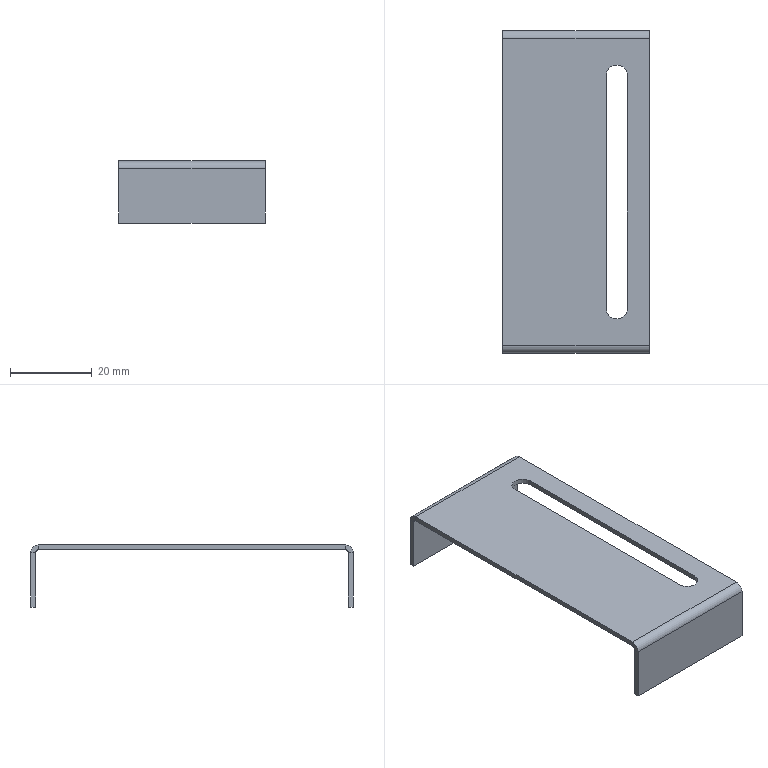Part | 1 solid | 26 faces | box 36 x 79 x 15.2 mm | volume 4192 mm3 | plane 20 | cylinder 6 | commonest cylinder face diameters 1.473 x2 3.873 x2 5.2 x2
STEP:
#1=CARTESIAN_POINT('',(12.6,-28.5,-1.2));
#2=VERTEX_POINT('',#1);
#3=CARTESIAN_POINT('',(7.4,-28.5,-1.2));
#4=VERTEX_POINT('',#3);
#5=CARTESIAN_POINT('',(10.,-28.5,-1.2));
#6=DIRECTION('',(0.,0.,-1.));
#7=DIRECTION('',(-1.,0.,0.));
#8=AXIS2_PLACEMENT_3D('',#5,#6,#7);
#9=CIRCLE('',#8,2.6);
#10=EDGE_CURVE('',#2,#4,#9,.T.);
#11=ORIENTED_EDGE('',*,*,#10,.F.);
#12=CARTESIAN_POINT('',(12.6,28.5,-1.2));
#13=VERTEX_POINT('',#12);
#14=CARTESIAN_POINT('',(12.6,-28.5,-1.2));
#15=DIRECTION('',(0.,-1.,0.));
#16=VECTOR('',#15,1000.);
#17=LINE('',#14,#16);
#18=EDGE_CURVE('',#13,#2,#17,.T.);
#19=ORIENTED_EDGE('',*,*,#18,.F.);
#20=CARTESIAN_POINT('',(7.4,28.5,-1.2));
#21=VERTEX_POINT('',#20);
#22=CARTESIAN_POINT('',(10.,28.5,-1.2));
#23=DIRECTION('',(0.,0.,-1.));
#24=DIRECTION('',(-1.,0.,0.));
#25=AXIS2_PLACEMENT_3D('',#22,#23,#24);
#26=CIRCLE('',#25,2.6);
#27=EDGE_CURVE('',#21,#13,#26,.T.);
#28=ORIENTED_EDGE('',*,*,#27,.F.);
#29=CARTESIAN_POINT('',(7.4,-28.5,-1.2));
#30=DIRECTION('',(0.,1.,0.));
#31=VECTOR('',#30,1000.);
#32=LINE('',#29,#31);
#33=EDGE_CURVE('',#4,#21,#32,.T.);
#34=ORIENTED_EDGE('',*,*,#33,.F.);
#35=EDGE_LOOP('',(#11,#19,#28,#34));
#36=FACE_BOUND('',#35,.T.);
#37=CARTESIAN_POINT('',(18.,-37.563,-1.2));
#38=VERTEX_POINT('',#37);
#39=CARTESIAN_POINT('',(18.,37.563,-1.2));
#40=VERTEX_POINT('',#39);
#41=CARTESIAN_POINT('',(18.,-39.5,-1.2));
#42=DIRECTION('',(0.,1.,0.));
#43=VECTOR('',#42,1000.);
#44=LINE('',#41,#43);
#45=EDGE_CURVE('',#38,#40,#44,.T.);
#46=ORIENTED_EDGE('',*,*,#45,.F.);
#47=CARTESIAN_POINT('',(-18.,-37.563,-1.2));
#48=VERTEX_POINT('',#47);
#49=CARTESIAN_POINT('',(-18.,-37.563,-1.2));
#50=DIRECTION('',(1.,0.,0.));
#51=VECTOR('',#50,1000.);
#52=LINE('',#49,#51);
#53=EDGE_CURVE('',#48,#38,#52,.T.);
#54=ORIENTED_EDGE('',*,*,#53,.F.);
#55=CARTESIAN_POINT('',(-18.,37.563,-1.2));
#56=VERTEX_POINT('',#55);
#57=CARTESIAN_POINT('',(-18.,-39.5,-1.2));
#58=DIRECTION('',(0.,-1.,0.));
#59=VECTOR('',#58,1000.);
#60=LINE('',#57,#59);
#61=EDGE_CURVE('',#56,#48,#60,.T.);
#62=ORIENTED_EDGE('',*,*,#61,.F.);
#63=CARTESIAN_POINT('',(18.,37.563,-1.2));
#64=DIRECTION('',(-1.,0.,0.));
#65=VECTOR('',#64,1000.);
#66=LINE('',#63,#65);
#67=EDGE_CURVE('',#40,#56,#66,.T.);
#68=ORIENTED_EDGE('',*,*,#67,.F.);
#69=EDGE_LOOP('',(#46,#54,#62,#68));
#70=FACE_OUTER_BOUND('',#69,.T.);
#71=CARTESIAN_POINT('',(0.,0.,-1.2));
#72=DIRECTION('',(0.,0.,-1.));
#73=DIRECTION('',(-1.,0.,0.));
#74=AXIS2_PLACEMENT_3D('',#71,#72,#73);
#75=PLANE('',#74);
#76=ADVANCED_FACE('',(#36,#70),#75,.T.);
#77=CARTESIAN_POINT('',(12.6,28.5,0.));
#78=VERTEX_POINT('',#77);
#79=CARTESIAN_POINT('',(12.6,-28.5,0.));
#80=VERTEX_POINT('',#79);
#81=CARTESIAN_POINT('',(12.6,0.,0.));
#82=DIRECTION('',(0.,-1.,0.));
#83=VECTOR('',#82,1000.);
#84=LINE('',#81,#83);
#85=EDGE_CURVE('',#78,#80,#84,.T.);
#86=ORIENTED_EDGE('',*,*,#85,.T.);
#87=CARTESIAN_POINT('',(7.4,-28.5,0.));
#88=VERTEX_POINT('',#87);
#89=CARTESIAN_POINT('',(10.,-28.5,0.));
#90=DIRECTION('',(0.,0.,-1.));
#91=DIRECTION('',(-1.,0.,0.));
#92=AXIS2_PLACEMENT_3D('',#89,#90,#91);
#93=CIRCLE('',#92,2.6);
#94=EDGE_CURVE('',#80,#88,#93,.T.);
#95=ORIENTED_EDGE('',*,*,#94,.T.);
#96=CARTESIAN_POINT('',(7.4,28.5,0.));
#97=VERTEX_POINT('',#96);
#98=CARTESIAN_POINT('',(7.4,0.,0.));
#99=DIRECTION('',(0.,1.,0.));
#100=VECTOR('',#99,1000.);
#101=LINE('',#98,#100);
#102=EDGE_CURVE('',#88,#97,#101,.T.);
#103=ORIENTED_EDGE('',*,*,#102,.T.);
#104=CARTESIAN_POINT('',(10.,28.5,0.));
#105=DIRECTION('',(0.,0.,-1.));
#106=DIRECTION('',(-1.,0.,0.));
#107=AXIS2_PLACEMENT_3D('',#104,#105,#106);
#108=CIRCLE('',#107,2.6);
#109=EDGE_CURVE('',#97,#78,#108,.T.);
#110=ORIENTED_EDGE('',*,*,#109,.T.);
#111=EDGE_LOOP('',(#86,#95,#103,#110));
#112=FACE_BOUND('',#111,.T.);
#113=CARTESIAN_POINT('',(-18.,-37.563,0.));
#114=VERTEX_POINT('',#113);
#115=CARTESIAN_POINT('',(18.,-37.563,0.));
#116=VERTEX_POINT('',#115);
#117=CARTESIAN_POINT('',(-18.,-37.563,0.));
#118=DIRECTION('',(1.,0.,0.));
#119=VECTOR('',#118,1000.);
#120=LINE('',#117,#119);
#121=EDGE_CURVE('',#114,#116,#120,.T.);
#122=ORIENTED_EDGE('',*,*,#121,.T.);
#123=CARTESIAN_POINT('',(18.,37.563,0.));
#124=VERTEX_POINT('',#123);
#125=CARTESIAN_POINT('',(18.,-39.5,0.));
#126=DIRECTION('',(0.,1.,0.));
#127=VECTOR('',#126,1000.);
#128=LINE('',#125,#127);
#129=EDGE_CURVE('',#116,#124,#128,.T.);
#130=ORIENTED_EDGE('',*,*,#129,.T.);
#131=CARTESIAN_POINT('',(-18.,37.563,0.));
#132=VERTEX_POINT('',#131);
#133=CARTESIAN_POINT('',(18.,37.563,0.));
#134=DIRECTION('',(-1.,0.,0.));
#135=VECTOR('',#134,1000.);
#136=LINE('',#133,#135);
#137=EDGE_CURVE('',#124,#132,#136,.T.);
#138=ORIENTED_EDGE('',*,*,#137,.T.);
#139=CARTESIAN_POINT('',(-18.,-39.5,0.));
#140=DIRECTION('',(0.,-1.,0.));
#141=VECTOR('',#140,1000.);
#142=LINE('',#139,#141);
#143=EDGE_CURVE('',#132,#114,#142,.T.);
#144=ORIENTED_EDGE('',*,*,#143,.T.);
#145=EDGE_LOOP('',(#122,#130,#138,#144));
#146=FACE_OUTER_BOUND('',#145,.T.);
#147=CARTESIAN_POINT('',(0.,0.,0.));
#148=DIRECTION('',(0.,0.,-1.));
#149=DIRECTION('',(-1.,0.,0.));
#150=AXIS2_PLACEMENT_3D('',#147,#148,#149);
#151=PLANE('',#150);
#152=ADVANCED_FACE('',(#112,#146),#151,.F.);
#153=ORIENTED_EDGE('',*,*,#61,.T.);
#154=CARTESIAN_POINT('',(-18.,-37.563,-1.2));
#155=DIRECTION('',(0.,0.,1.));
#156=VECTOR('',#155,1000.);
#157=LINE('',#154,#156);
#158=EDGE_CURVE('',#48,#114,#157,.T.);
#159=ORIENTED_EDGE('',*,*,#158,.T.);
#160=ORIENTED_EDGE('',*,*,#143,.F.);
#161=CARTESIAN_POINT('',(-18.,37.563,-1.2));
#162=DIRECTION('',(0.,0.,1.));
#163=VECTOR('',#162,1000.);
#164=LINE('',#161,#163);
#165=EDGE_CURVE('',#56,#132,#164,.T.);
#166=ORIENTED_EDGE('',*,*,#165,.F.);
#167=EDGE_LOOP('',(#153,#159,#160,#166));
#168=FACE_OUTER_BOUND('',#167,.T.);
#169=CARTESIAN_POINT('',(-18.,-39.5,-1.2));
#170=DIRECTION('',(-1.,0.,0.));
#171=DIRECTION('',(0.,0.,1.));
#172=AXIS2_PLACEMENT_3D('',#169,#170,#171);
#173=PLANE('',#172);
#174=ADVANCED_FACE('',(#168),#173,.T.);
#175=CARTESIAN_POINT('',(18.,-37.563,-1.2));
#176=DIRECTION('',(0.,0.,1.));
#177=VECTOR('',#176,1000.);
#178=LINE('',#175,#177);
#179=EDGE_CURVE('',#38,#116,#178,.T.);
#180=ORIENTED_EDGE('',*,*,#179,.F.);
#181=ORIENTED_EDGE('',*,*,#45,.T.);
#182=CARTESIAN_POINT('',(18.,37.563,-1.2));
#183=DIRECTION('',(0.,0.,1.));
#184=VECTOR('',#183,1000.);
#185=LINE('',#182,#184);
#186=EDGE_CURVE('',#40,#124,#185,.T.);
#187=ORIENTED_EDGE('',*,*,#186,.T.);
#188=ORIENTED_EDGE('',*,*,#129,.F.);
#189=EDGE_LOOP('',(#180,#181,#187,#188));
#190=FACE_OUTER_BOUND('',#189,.T.);
#191=CARTESIAN_POINT('',(18.,-39.5,-1.2));
#192=DIRECTION('',(1.,0.,0.));
#193=DIRECTION('',(0.,0.,-1.));
#194=AXIS2_PLACEMENT_3D('',#191,#192,#193);
#195=PLANE('',#194);
#196=ADVANCED_FACE('',(#190),#195,.T.);
#197=CARTESIAN_POINT('',(-18.,38.3,-1.937));
#198=VERTEX_POINT('',#197);
#199=CARTESIAN_POINT('',(-18.,39.5,-1.937));
#200=VERTEX_POINT('',#199);
#201=CARTESIAN_POINT('',(-18.,39.5,-1.937));
#202=DIRECTION('',(0.,1.,0.));
#203=VECTOR('',#202,1000.);
#204=LINE('',#201,#203);
#205=EDGE_CURVE('',#198,#200,#204,.T.);
#206=ORIENTED_EDGE('',*,*,#205,.F.);
#207=CARTESIAN_POINT('',(-18.,37.563,-1.937));
#208=DIRECTION('',(-1.,0.,0.));
#209=DIRECTION('',(0.,0.,-1.));
#210=AXIS2_PLACEMENT_3D('',#207,#208,#209);
#211=CIRCLE('',#210,0.7366);
#212=EDGE_CURVE('',#56,#198,#211,.T.);
#213=ORIENTED_EDGE('',*,*,#212,.F.);
#214=ORIENTED_EDGE('',*,*,#165,.T.);
#215=CARTESIAN_POINT('',(-18.,37.563,-1.937));
#216=DIRECTION('',(-1.,0.,0.));
#217=DIRECTION('',(0.,0.,-1.));
#218=AXIS2_PLACEMENT_3D('',#215,#216,#217);
#219=CIRCLE('',#218,1.937);
#220=EDGE_CURVE('',#132,#200,#219,.T.);
#221=ORIENTED_EDGE('',*,*,#220,.T.);
#222=EDGE_LOOP('',(#206,#213,#214,#221));
#223=FACE_OUTER_BOUND('',#222,.T.);
#224=CARTESIAN_POINT('',(-18.,37.563,-1.937));
#225=DIRECTION('',(-1.,0.,0.));
#226=DIRECTION('',(0.,0.,1.));
#227=AXIS2_PLACEMENT_3D('',#224,#225,#226);
#228=PLANE('',#227);
#229=ADVANCED_FACE('',(#223),#228,.T.);
#230=CARTESIAN_POINT('',(18.,38.3,-1.937));
#231=VERTEX_POINT('',#230);
#232=CARTESIAN_POINT('',(18.,37.563,-1.937));
#233=DIRECTION('',(1.,0.,0.));
#234=DIRECTION('',(0.,0.,-1.));
#235=AXIS2_PLACEMENT_3D('',#232,#233,#234);
#236=CIRCLE('',#235,0.7366);
#237=EDGE_CURVE('',#231,#40,#236,.T.);
#238=ORIENTED_EDGE('',*,*,#237,.F.);
#239=CARTESIAN_POINT('',(18.,39.5,-1.937));
#240=VERTEX_POINT('',#239);
#241=CARTESIAN_POINT('',(18.,38.3,-1.937));
#242=DIRECTION('',(0.,1.,0.));
#243=VECTOR('',#242,1000.);
#244=LINE('',#241,#243);
#245=EDGE_CURVE('',#231,#240,#244,.T.);
#246=ORIENTED_EDGE('',*,*,#245,.T.);
#247=CARTESIAN_POINT('',(18.,37.563,-1.937));
#248=DIRECTION('',(1.,0.,0.));
#249=DIRECTION('',(0.,0.,-1.));
#250=AXIS2_PLACEMENT_3D('',#247,#248,#249);
#251=CIRCLE('',#250,1.937);
#252=EDGE_CURVE('',#240,#124,#251,.T.);
#253=ORIENTED_EDGE('',*,*,#252,.T.);
#254=ORIENTED_EDGE('',*,*,#186,.F.);
#255=EDGE_LOOP('',(#238,#246,#253,#254));
#256=FACE_OUTER_BOUND('',#255,.T.);
#257=CARTESIAN_POINT('',(18.,37.563,-1.937));
#258=DIRECTION('',(-1.,0.,0.));
#259=DIRECTION('',(0.,0.,1.));
#260=AXIS2_PLACEMENT_3D('',#257,#258,#259);
#261=PLANE('',#260);
#262=ADVANCED_FACE('',(#256),#261,.F.);
#263=ORIENTED_EDGE('',*,*,#137,.F.);
#264=ORIENTED_EDGE('',*,*,#252,.F.);
#265=CARTESIAN_POINT('',(0.,39.5,-1.937));
#266=DIRECTION('',(1.,0.,0.));
#267=VECTOR('',#266,1000.);
#268=LINE('',#265,#267);
#269=EDGE_CURVE('',#200,#240,#268,.T.);
#270=ORIENTED_EDGE('',*,*,#269,.F.);
#271=ORIENTED_EDGE('',*,*,#220,.F.);
#272=EDGE_LOOP('',(#263,#264,#270,#271));
#273=FACE_OUTER_BOUND('',#272,.T.);
#274=CARTESIAN_POINT('',(18.,37.563,-1.937));
#275=DIRECTION('',(1.,0.,0.));
#276=DIRECTION('',(0.,1.,0.));
#277=AXIS2_PLACEMENT_3D('',#274,#275,#276);
#278=CYLINDRICAL_SURFACE('',#277,1.937);
#279=ADVANCED_FACE('',(#273),#278,.T.);
#280=ORIENTED_EDGE('',*,*,#67,.T.);
#281=ORIENTED_EDGE('',*,*,#212,.T.);
#282=CARTESIAN_POINT('',(-18.,38.3,-1.937));
#283=DIRECTION('',(1.,0.,0.));
#284=VECTOR('',#283,1000.);
#285=LINE('',#282,#284);
#286=EDGE_CURVE('',#198,#231,#285,.T.);
#287=ORIENTED_EDGE('',*,*,#286,.T.);
#288=ORIENTED_EDGE('',*,*,#237,.T.);
#289=EDGE_LOOP('',(#280,#281,#287,#288));
#290=FACE_OUTER_BOUND('',#289,.T.);
#291=CARTESIAN_POINT('',(18.,37.563,-1.937));
#292=DIRECTION('',(1.,0.,0.));
#293=DIRECTION('',(0.,1.,0.));
#294=AXIS2_PLACEMENT_3D('',#291,#292,#293);
#295=CYLINDRICAL_SURFACE('',#294,0.7366);
#296=ADVANCED_FACE('',(#290),#295,.F.);
#297=CARTESIAN_POINT('',(18.,39.5,-15.2));
#298=VERTEX_POINT('',#297);
#299=CARTESIAN_POINT('',(18.,39.5,-1.2));
#300=DIRECTION('',(0.,0.,1.));
#301=VECTOR('',#300,1000.);
#302=LINE('',#299,#301);
#303=EDGE_CURVE('',#298,#240,#302,.T.);
#304=ORIENTED_EDGE('',*,*,#303,.T.);
#305=ORIENTED_EDGE('',*,*,#245,.F.);
#306=CARTESIAN_POINT('',(18.,38.3,-15.2));
#307=VERTEX_POINT('',#306);
#308=CARTESIAN_POINT('',(18.,38.3,0.));
#309=DIRECTION('',(0.,0.,1.));
#310=VECTOR('',#309,1000.);
#311=LINE('',#308,#310);
#312=EDGE_CURVE('',#307,#231,#311,.T.);
#313=ORIENTED_EDGE('',*,*,#312,.F.);
#314=CARTESIAN_POINT('',(18.,39.5,-15.2));
#315=DIRECTION('',(0.,-1.,0.));
#316=VECTOR('',#315,1000.);
#317=LINE('',#314,#316);
#318=EDGE_CURVE('',#298,#307,#317,.T.);
#319=ORIENTED_EDGE('',*,*,#318,.F.);
#320=EDGE_LOOP('',(#304,#305,#313,#319));
#321=FACE_OUTER_BOUND('',#320,.T.);
#322=CARTESIAN_POINT('',(18.,39.5,-1.2));
#323=DIRECTION('',(1.,0.,0.));
#324=DIRECTION('',(0.,0.,-1.));
#325=AXIS2_PLACEMENT_3D('',#322,#323,#324);
#326=PLANE('',#325);
#327=ADVANCED_FACE('',(#321),#326,.T.);
#328=CARTESIAN_POINT('',(-18.,38.3,-15.2));
#329=VERTEX_POINT('',#328);
#330=CARTESIAN_POINT('',(-18.,38.3,0.));
#331=DIRECTION('',(0.,0.,-1.));
#332=VECTOR('',#331,1000.);
#333=LINE('',#330,#332);
#334=EDGE_CURVE('',#198,#329,#333,.T.);
#335=ORIENTED_EDGE('',*,*,#334,.F.);
#336=ORIENTED_EDGE('',*,*,#205,.T.);
#337=CARTESIAN_POINT('',(-18.,39.5,-15.2));
#338=VERTEX_POINT('',#337);
#339=CARTESIAN_POINT('',(-18.,39.5,-15.2));
#340=DIRECTION('',(0.,0.,-1.));
#341=VECTOR('',#340,1000.);
#342=LINE('',#339,#341);
#343=EDGE_CURVE('',#200,#338,#342,.T.);
#344=ORIENTED_EDGE('',*,*,#343,.T.);
#345=CARTESIAN_POINT('',(-18.,39.5,-15.2));
#346=DIRECTION('',(0.,-1.,0.));
#347=VECTOR('',#346,1000.);
#348=LINE('',#345,#347);
#349=EDGE_CURVE('',#338,#329,#348,.T.);
#350=ORIENTED_EDGE('',*,*,#349,.T.);
#351=EDGE_LOOP('',(#335,#336,#344,#350));
#352=FACE_OUTER_BOUND('',#351,.T.);
#353=CARTESIAN_POINT('',(-18.,39.5,-15.2));
#354=DIRECTION('',(-1.,0.,0.));
#355=DIRECTION('',(0.,0.,1.));
#356=AXIS2_PLACEMENT_3D('',#353,#354,#355);
#357=PLANE('',#356);
#358=ADVANCED_FACE('',(#352),#357,.T.);
#359=ORIENTED_EDGE('',*,*,#343,.F.);
#360=ORIENTED_EDGE('',*,*,#269,.T.);
#361=ORIENTED_EDGE('',*,*,#303,.F.);
#362=CARTESIAN_POINT('',(18.,39.5,-15.2));
#363=DIRECTION('',(1.,0.,0.));
#364=VECTOR('',#363,1000.);
#365=LINE('',#362,#364);
#366=EDGE_CURVE('',#338,#298,#365,.T.);
#367=ORIENTED_EDGE('',*,*,#366,.F.);
#368=EDGE_LOOP('',(#359,#360,#361,#367));
#369=FACE_OUTER_BOUND('',#368,.T.);
#370=CARTESIAN_POINT('',(0.,39.5,0.));
#371=DIRECTION('',(0.,1.,0.));
#372=DIRECTION('',(0.,0.,1.));
#373=AXIS2_PLACEMENT_3D('',#370,#371,#372);
#374=PLANE('',#373);
#375=ADVANCED_FACE('',(#369),#374,.T.);
#376=ORIENTED_EDGE('',*,*,#286,.F.);
#377=ORIENTED_EDGE('',*,*,#334,.T.);
#378=CARTESIAN_POINT('',(0.,38.3,-15.2));
#379=DIRECTION('',(1.,0.,0.));
#380=VECTOR('',#379,1000.);
#381=LINE('',#378,#380);
#382=EDGE_CURVE('',#329,#307,#381,.T.);
#383=ORIENTED_EDGE('',*,*,#382,.T.);
#384=ORIENTED_EDGE('',*,*,#312,.T.);
#385=EDGE_LOOP('',(#376,#377,#383,#384));
#386=FACE_OUTER_BOUND('',#385,.T.);
#387=CARTESIAN_POINT('',(0.,38.3,0.));
#388=DIRECTION('',(0.,1.,0.));
#389=DIRECTION('',(0.,0.,1.));
#390=AXIS2_PLACEMENT_3D('',#387,#388,#389);
#391=PLANE('',#390);
#392=ADVANCED_FACE('',(#386),#391,.F.);
#393=ORIENTED_EDGE('',*,*,#382,.F.);
#394=ORIENTED_EDGE('',*,*,#349,.F.);
#395=ORIENTED_EDGE('',*,*,#366,.T.);
#396=ORIENTED_EDGE('',*,*,#318,.T.);
#397=EDGE_LOOP('',(#393,#394,#395,#396));
#398=FACE_OUTER_BOUND('',#397,.T.);
#399=CARTESIAN_POINT('',(18.,39.5,-15.2));
#400=DIRECTION('',(0.,0.,-1.));
#401=DIRECTION('',(0.,1.,0.));
#402=AXIS2_PLACEMENT_3D('',#399,#400,#401);
#403=PLANE('',#402);
#404=ADVANCED_FACE('',(#398),#403,.T.);
#405=CARTESIAN_POINT('',(18.,-38.3,-1.937));
#406=VERTEX_POINT('',#405);
#407=CARTESIAN_POINT('',(18.,-39.5,-1.937));
#408=VERTEX_POINT('',#407);
#409=CARTESIAN_POINT('',(18.,-39.5,-1.937));
#410=DIRECTION('',(0.,-1.,0.));
#411=VECTOR('',#410,1000.);
#412=LINE('',#409,#411);
#413=EDGE_CURVE('',#406,#408,#412,.T.);
#414=ORIENTED_EDGE('',*,*,#413,.F.);
#415=CARTESIAN_POINT('',(18.,-37.563,-1.937));
#416=DIRECTION('',(1.,0.,0.));
#417=DIRECTION('',(0.,0.,1.));
#418=AXIS2_PLACEMENT_3D('',#415,#416,#417);
#419=CIRCLE('',#418,0.7366);
#420=EDGE_CURVE('',#38,#406,#419,.T.);
#421=ORIENTED_EDGE('',*,*,#420,.F.);
#422=ORIENTED_EDGE('',*,*,#179,.T.);
#423=CARTESIAN_POINT('',(18.,-37.563,-1.937));
#424=DIRECTION('',(1.,0.,0.));
#425=DIRECTION('',(0.,0.,1.));
#426=AXIS2_PLACEMENT_3D('',#423,#424,#425);
#427=CIRCLE('',#426,1.937);
#428=EDGE_CURVE('',#116,#408,#427,.T.);
#429=ORIENTED_EDGE('',*,*,#428,.T.);
#430=EDGE_LOOP('',(#414,#421,#422,#429));
#431=FACE_OUTER_BOUND('',#430,.T.);
#432=CARTESIAN_POINT('',(18.,-37.563,-1.937));
#433=DIRECTION('',(1.,0.,0.));
#434=DIRECTION('',(0.,0.,-1.));
#435=AXIS2_PLACEMENT_3D('',#432,#433,#434);
#436=PLANE('',#435);
#437=ADVANCED_FACE('',(#431),#436,.T.);
#438=CARTESIAN_POINT('',(-18.,-38.3,-1.937));
#439=VERTEX_POINT('',#438);
#440=CARTESIAN_POINT('',(-18.,-37.563,-1.937));
#441=DIRECTION('',(-1.,0.,0.));
#442=DIRECTION('',(0.,0.,1.));
#443=AXIS2_PLACEMENT_3D('',#440,#441,#442);
#444=CIRCLE('',#443,0.7366);
#445=EDGE_CURVE('',#439,#48,#444,.T.);
#446=ORIENTED_EDGE('',*,*,#445,.F.);
#447=CARTESIAN_POINT('',(-18.,-39.5,-1.937));
#448=VERTEX_POINT('',#447);
#449=CARTESIAN_POINT('',(-18.,-38.3,-1.937));
#450=DIRECTION('',(0.,-1.,0.));
#451=VECTOR('',#450,1000.);
#452=LINE('',#449,#451);
#453=EDGE_CURVE('',#439,#448,#452,.T.);
#454=ORIENTED_EDGE('',*,*,#453,.T.);
#455=CARTESIAN_POINT('',(-18.,-37.563,-1.937));
#456=DIRECTION('',(-1.,0.,0.));
#457=DIRECTION('',(0.,0.,1.));
#458=AXIS2_PLACEMENT_3D('',#455,#456,#457);
#459=CIRCLE('',#458,1.937);
#460=EDGE_CURVE('',#448,#114,#459,.T.);
#461=ORIENTED_EDGE('',*,*,#460,.T.);
#462=ORIENTED_EDGE('',*,*,#158,.F.);
#463=EDGE_LOOP('',(#446,#454,#461,#462));
#464=FACE_OUTER_BOUND('',#463,.T.);
#465=CARTESIAN_POINT('',(-18.,-37.563,-1.937));
#466=DIRECTION('',(1.,0.,0.));
#467=DIRECTION('',(0.,0.,-1.));
#468=AXIS2_PLACEMENT_3D('',#465,#466,#467);
#469=PLANE('',#468);
#470=ADVANCED_FACE('',(#464),#469,.F.);
#471=ORIENTED_EDGE('',*,*,#121,.F.);
#472=ORIENTED_EDGE('',*,*,#460,.F.);
#473=CARTESIAN_POINT('',(18.,-39.5,-1.937));
#474=DIRECTION('',(1.,0.,0.));
#475=VECTOR('',#474,1000.);
#476=LINE('',#473,#475);
#477=EDGE_CURVE('',#448,#408,#476,.T.);
#478=ORIENTED_EDGE('',*,*,#477,.T.);
#479=ORIENTED_EDGE('',*,*,#428,.F.);
#480=EDGE_LOOP('',(#471,#472,#478,#479));
#481=FACE_OUTER_BOUND('',#480,.T.);
#482=CARTESIAN_POINT('',(-18.,-37.563,-1.937));
#483=DIRECTION('',(-1.,0.,0.));
#484=DIRECTION('',(0.,-1.,0.));
#485=AXIS2_PLACEMENT_3D('',#482,#483,#484);
#486=CYLINDRICAL_SURFACE('',#485,1.937);
#487=ADVANCED_FACE('',(#481),#486,.T.);
#488=ORIENTED_EDGE('',*,*,#53,.T.);
#489=ORIENTED_EDGE('',*,*,#420,.T.);
#490=CARTESIAN_POINT('',(18.,-38.3,-1.937));
#491=DIRECTION('',(-1.,0.,0.));
#492=VECTOR('',#491,1000.);
#493=LINE('',#490,#492);
#494=EDGE_CURVE('',#406,#439,#493,.T.);
#495=ORIENTED_EDGE('',*,*,#494,.T.);
#496=ORIENTED_EDGE('',*,*,#445,.T.);
#497=EDGE_LOOP('',(#488,#489,#495,#496));
#498=FACE_OUTER_BOUND('',#497,.T.);
#499=CARTESIAN_POINT('',(-18.,-37.563,-1.937));
#500=DIRECTION('',(-1.,0.,0.));
#501=DIRECTION('',(0.,-1.,0.));
#502=AXIS2_PLACEMENT_3D('',#499,#500,#501);
#503=CYLINDRICAL_SURFACE('',#502,0.7366);
#504=ADVANCED_FACE('',(#498),#503,.F.);
#505=CARTESIAN_POINT('',(18.,-38.3,-15.2));
#506=VERTEX_POINT('',#505);
#507=CARTESIAN_POINT('',(18.,-38.3,0.));
#508=DIRECTION('',(0.,0.,-1.));
#509=VECTOR('',#508,1000.);
#510=LINE('',#507,#509);
#511=EDGE_CURVE('',#406,#506,#510,.T.);
#512=ORIENTED_EDGE('',*,*,#511,.F.);
#513=ORIENTED_EDGE('',*,*,#413,.T.);
#514=CARTESIAN_POINT('',(18.,-39.5,-15.2));
#515=VERTEX_POINT('',#514);
#516=CARTESIAN_POINT('',(18.,-39.5,-1.2));
#517=DIRECTION('',(0.,0.,-1.));
#518=VECTOR('',#517,1000.);
#519=LINE('',#516,#518);
#520=EDGE_CURVE('',#408,#515,#519,.T.);
#521=ORIENTED_EDGE('',*,*,#520,.T.);
#522=CARTESIAN_POINT('',(18.,-39.5,-15.2));
#523=DIRECTION('',(0.,1.,0.));
#524=VECTOR('',#523,1000.);
#525=LINE('',#522,#524);
#526=EDGE_CURVE('',#515,#506,#525,.T.);
#527=ORIENTED_EDGE('',*,*,#526,.T.);
#528=EDGE_LOOP('',(#512,#513,#521,#527));
#529=FACE_OUTER_BOUND('',#528,.T.);
#530=CARTESIAN_POINT('',(18.,-39.5,-1.2));
#531=DIRECTION('',(1.,0.,0.));
#532=DIRECTION('',(0.,0.,-1.));
#533=AXIS2_PLACEMENT_3D('',#530,#531,#532);
#534=PLANE('',#533);
#535=ADVANCED_FACE('',(#529),#534,.T.);
#536=CARTESIAN_POINT('',(-18.,-39.5,-15.2));
#537=VERTEX_POINT('',#536);
#538=CARTESIAN_POINT('',(-18.,-39.5,-15.2));
#539=DIRECTION('',(0.,0.,1.));
#540=VECTOR('',#539,1000.);
#541=LINE('',#538,#540);
#542=EDGE_CURVE('',#537,#448,#541,.T.);
#543=ORIENTED_EDGE('',*,*,#542,.T.);
#544=ORIENTED_EDGE('',*,*,#453,.F.);
#545=CARTESIAN_POINT('',(-18.,-38.3,-15.2));
#546=VERTEX_POINT('',#545);
#547=CARTESIAN_POINT('',(-18.,-38.3,0.));
#548=DIRECTION('',(0.,0.,1.));
#549=VECTOR('',#548,1000.);
#550=LINE('',#547,#549);
#551=EDGE_CURVE('',#546,#439,#550,.T.);
#552=ORIENTED_EDGE('',*,*,#551,.F.);
#553=CARTESIAN_POINT('',(-18.,-39.5,-15.2));
#554=DIRECTION('',(0.,1.,0.));
#555=VECTOR('',#554,1000.);
#556=LINE('',#553,#555);
#557=EDGE_CURVE('',#537,#546,#556,.T.);
#558=ORIENTED_EDGE('',*,*,#557,.F.);
#559=EDGE_LOOP('',(#543,#544,#552,#558));
#560=FACE_OUTER_BOUND('',#559,.T.);
#561=CARTESIAN_POINT('',(-18.,-39.5,-15.2));
#562=DIRECTION('',(-1.,0.,0.));
#563=DIRECTION('',(0.,0.,1.));
#564=AXIS2_PLACEMENT_3D('',#561,#562,#563);
#565=PLANE('',#564);
#566=ADVANCED_FACE('',(#560),#565,.T.);
#567=ORIENTED_EDGE('',*,*,#477,.F.);
#568=ORIENTED_EDGE('',*,*,#542,.F.);
#569=CARTESIAN_POINT('',(18.,-39.5,-15.2));
#570=DIRECTION('',(-1.,0.,0.));
#571=VECTOR('',#570,1000.);
#572=LINE('',#569,#571);
#573=EDGE_CURVE('',#515,#537,#572,.T.);
#574=ORIENTED_EDGE('',*,*,#573,.F.);
#575=ORIENTED_EDGE('',*,*,#520,.F.);
#576=EDGE_LOOP('',(#567,#568,#574,#575));
#577=FACE_OUTER_BOUND('',#576,.T.);
#578=CARTESIAN_POINT('',(0.,-39.5,0.));
#579=DIRECTION('',(0.,1.,0.));
#580=DIRECTION('',(0.,0.,1.));
#581=AXIS2_PLACEMENT_3D('',#578,#579,#580);
#582=PLANE('',#581);
#583=ADVANCED_FACE('',(#577),#582,.F.);
#584=ORIENTED_EDGE('',*,*,#551,.T.);
#585=ORIENTED_EDGE('',*,*,#494,.F.);
#586=ORIENTED_EDGE('',*,*,#511,.T.);
#587=CARTESIAN_POINT('',(0.,-38.3,-15.2));
#588=DIRECTION('',(-1.,0.,0.));
#589=VECTOR('',#588,1000.);
#590=LINE('',#587,#589);
#591=EDGE_CURVE('',#506,#546,#590,.T.);
#592=ORIENTED_EDGE('',*,*,#591,.T.);
#593=EDGE_LOOP('',(#584,#585,#586,#592));
#594=FACE_OUTER_BOUND('',#593,.T.);
#595=CARTESIAN_POINT('',(0.,-38.3,0.));
#596=DIRECTION('',(0.,1.,0.));
#597=DIRECTION('',(0.,0.,1.));
#598=AXIS2_PLACEMENT_3D('',#595,#596,#597);
#599=PLANE('',#598);
#600=ADVANCED_FACE('',(#594),#599,.T.);
#601=ORIENTED_EDGE('',*,*,#591,.F.);
#602=ORIENTED_EDGE('',*,*,#526,.F.);
#603=ORIENTED_EDGE('',*,*,#573,.T.);
#604=ORIENTED_EDGE('',*,*,#557,.T.);
#605=EDGE_LOOP('',(#601,#602,#603,#604));
#606=FACE_OUTER_BOUND('',#605,.T.);
#607=CARTESIAN_POINT('',(18.,-39.5,-15.2));
#608=DIRECTION('',(0.,0.,-1.));
#609=DIRECTION('',(0.,1.,0.));
#610=AXIS2_PLACEMENT_3D('',#607,#608,#609);
#611=PLANE('',#610);
#612=ADVANCED_FACE('',(#606),#611,.T.);
#613=CARTESIAN_POINT('',(12.6,-28.5,8.8));
#614=DIRECTION('',(0.,0.,-1.));
#615=VECTOR('',#614,1000.);
#616=LINE('',#613,#615);
#617=EDGE_CURVE('',#80,#2,#616,.T.);
#618=ORIENTED_EDGE('',*,*,#617,.T.);
#619=ORIENTED_EDGE('',*,*,#10,.T.);
#620=CARTESIAN_POINT('',(7.4,-28.5,8.8));
#621=DIRECTION('',(0.,0.,-1.));
#622=VECTOR('',#621,1000.);
#623=LINE('',#620,#622);
#624=EDGE_CURVE('',#88,#4,#623,.T.);
#625=ORIENTED_EDGE('',*,*,#624,.F.);
#626=ORIENTED_EDGE('',*,*,#94,.F.);
#627=EDGE_LOOP('',(#618,#619,#625,#626));
#628=FACE_OUTER_BOUND('',#627,.T.);
#629=CARTESIAN_POINT('',(10.,-28.5,8.8));
#630=DIRECTION('',(0.,0.,-1.));
#631=DIRECTION('',(-1.,0.,0.));
#632=AXIS2_PLACEMENT_3D('',#629,#630,#631);
#633=CYLINDRICAL_SURFACE('',#632,2.6);
#634=ADVANCED_FACE('',(#628),#633,.F.);
#635=CARTESIAN_POINT('',(12.6,28.5,8.8));
#636=DIRECTION('',(0.,0.,-1.));
#637=VECTOR('',#636,1000.);
#638=LINE('',#635,#637);
#639=EDGE_CURVE('',#78,#13,#638,.T.);
#640=ORIENTED_EDGE('',*,*,#639,.T.);
#641=ORIENTED_EDGE('',*,*,#18,.T.);
#642=ORIENTED_EDGE('',*,*,#617,.F.);
#643=ORIENTED_EDGE('',*,*,#85,.F.);
#644=EDGE_LOOP('',(#640,#641,#642,#643));
#645=FACE_OUTER_BOUND('',#644,.T.);
#646=CARTESIAN_POINT('',(12.6,-28.5,8.8));
#647=DIRECTION('',(1.,0.,0.));
#648=DIRECTION('',(0.,0.,-1.));
#649=AXIS2_PLACEMENT_3D('',#646,#647,#648);
#650=PLANE('',#649);
#651=ADVANCED_FACE('',(#645),#650,.F.);
#652=CARTESIAN_POINT('',(7.4,28.5,8.8));
#653=DIRECTION('',(0.,0.,-1.));
#654=VECTOR('',#653,1000.);
#655=LINE('',#652,#654);
#656=EDGE_CURVE('',#97,#21,#655,.T.);
#657=ORIENTED_EDGE('',*,*,#656,.T.);
#658=ORIENTED_EDGE('',*,*,#27,.T.);
#659=ORIENTED_EDGE('',*,*,#639,.F.);
#660=ORIENTED_EDGE('',*,*,#109,.F.);
#661=EDGE_LOOP('',(#657,#658,#659,#660));
#662=FACE_OUTER_BOUND('',#661,.T.);
#663=CARTESIAN_POINT('',(10.,28.5,8.8));
#664=DIRECTION('',(0.,0.,-1.));
#665=DIRECTION('',(-1.,0.,0.));
#666=AXIS2_PLACEMENT_3D('',#663,#664,#665);
#667=CYLINDRICAL_SURFACE('',#666,2.6);
#668=ADVANCED_FACE('',(#662),#667,.F.);
#669=ORIENTED_EDGE('',*,*,#624,.T.);
#670=ORIENTED_EDGE('',*,*,#33,.T.);
#671=ORIENTED_EDGE('',*,*,#656,.F.);
#672=ORIENTED_EDGE('',*,*,#102,.F.);
#673=EDGE_LOOP('',(#669,#670,#671,#672));
#674=FACE_OUTER_BOUND('',#673,.T.);
#675=CARTESIAN_POINT('',(7.4,-28.5,8.8));
#676=DIRECTION('',(-1.,0.,0.));
#677=DIRECTION('',(0.,0.,1.));
#678=AXIS2_PLACEMENT_3D('',#675,#676,#677);
#679=PLANE('',#678);
#680=ADVANCED_FACE('',(#674),#679,.F.);
#681=CLOSED_SHELL('',(#76,#152,#174,#196,#229,#262,#279,#296,#327,#358,#375,#392,#404,#437,#470,#487,#504,#535,#566,#583,#600,#612,#634,#651,#668,#680));
#682=MANIFOLD_SOLID_BREP('',#681);
#683=CARTESIAN_POINT('',(0.,0.,0.));
#684=DIRECTION('',(0.,0.,1.));
#685=DIRECTION('',(1.,0.,0.));
#686=AXIS2_PLACEMENT_3D('',#683,#684,#685);
#687=(LENGTH_UNIT()NAMED_UNIT(*)SI_UNIT(.MILLI.,.METRE.));
#688=UNCERTAINTY_MEASURE_WITH_UNIT(LENGTH_MEASURE(0.00001),#687,'','');
#689=(NAMED_UNIT(*)PLANE_ANGLE_UNIT()SI_UNIT($,.RADIAN.));
#690=(NAMED_UNIT(*)SI_UNIT($,.STERADIAN.)SOLID_ANGLE_UNIT());
#691=(GEOMETRIC_REPRESENTATION_CONTEXT(3)GLOBAL_UNCERTAINTY_ASSIGNED_CONTEXT((#688))GLOBAL_UNIT_ASSIGNED_CONTEXT((#687,#689,#690))REPRESENTATION_CONTEXT('',''));
#692=ADVANCED_BREP_SHAPE_REPRESENTATION('',(#682,#686),#691);